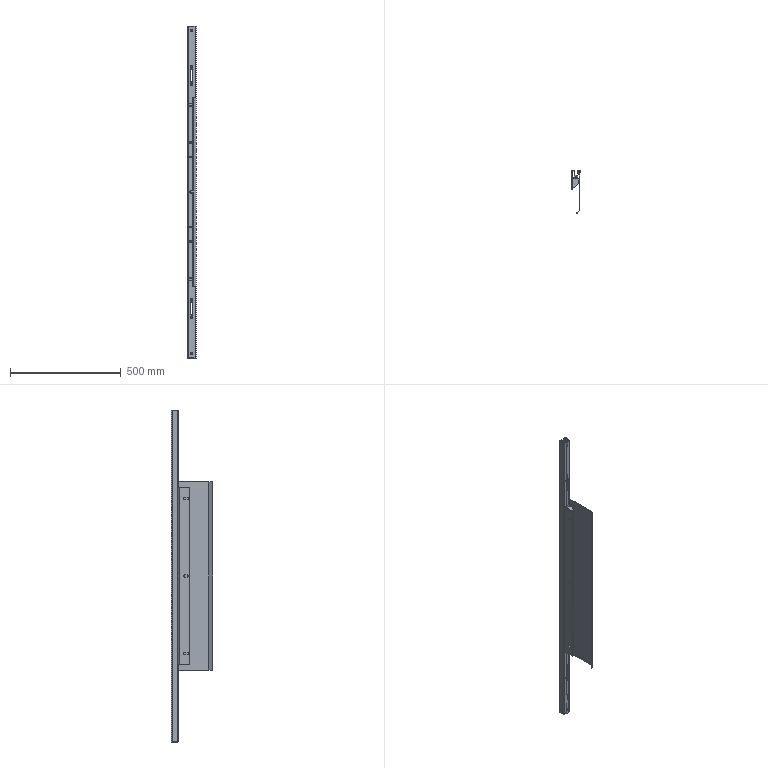Part | SolidWorks | 8 solids | 274 faces | box 40 x 188.321 x 1500 mm | volume 981117 mm3 | plane 177 | cylinder 97 | commonest cylinder face diameters 6 x23 10 x23 9 x15 2 x12 11 x12 10.5 x6